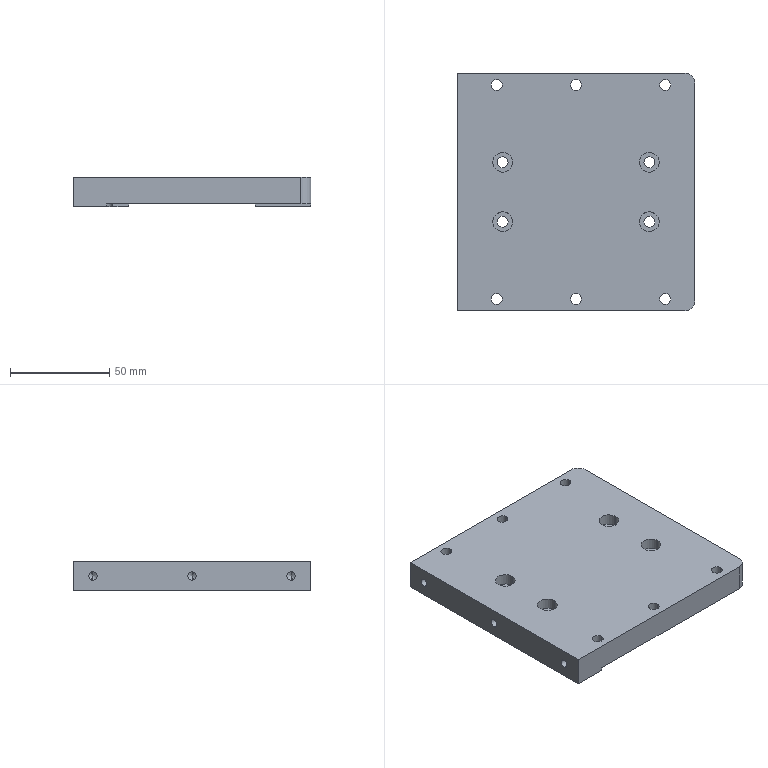Part | STEP file | PN_0014 | 1 solid | 79 faces | box 120 x 120 x 15 mm | volume 192156 mm3 | cylinder 49 | plane 24 | cone 6 | commonest cylinder face diameters 10 x22 5.5 x20 4.2 x6 6 x1